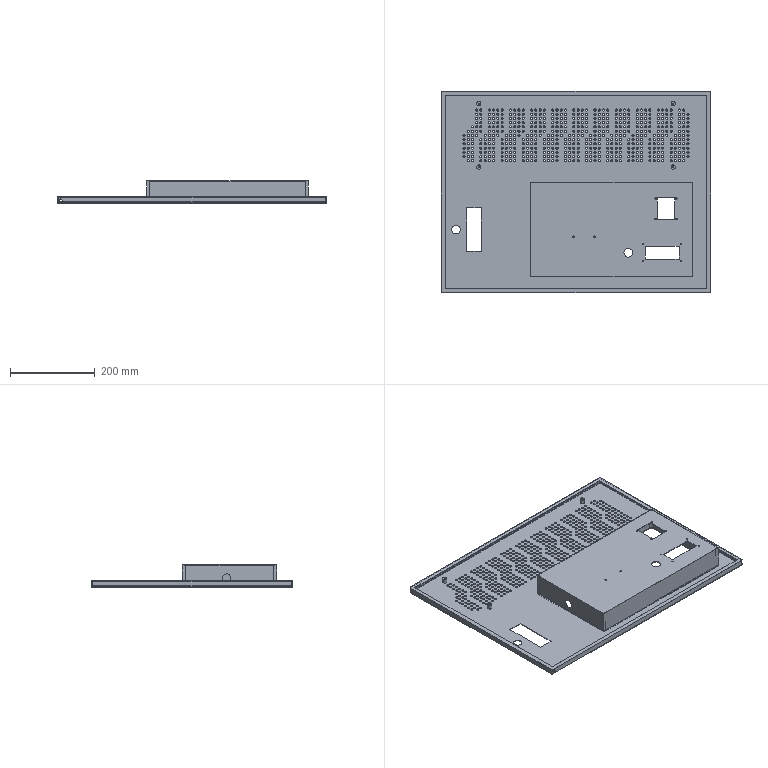Part | SolidWorks | features ICE 16, Fillet 4, HoleWzd 4, LPattern 4, Cut 1, Extrusion 1 | 5 solids | 1240 faces | box 638 x 478 x 53 mm | volume 589173 mm3 | cylinder 1178 | plane 46 | cone 8 | torus 8 | commonest cylinder face diameters 5 x1108 3.3 x16 2.5 x8 4.5 x8 6 x8 10 x8